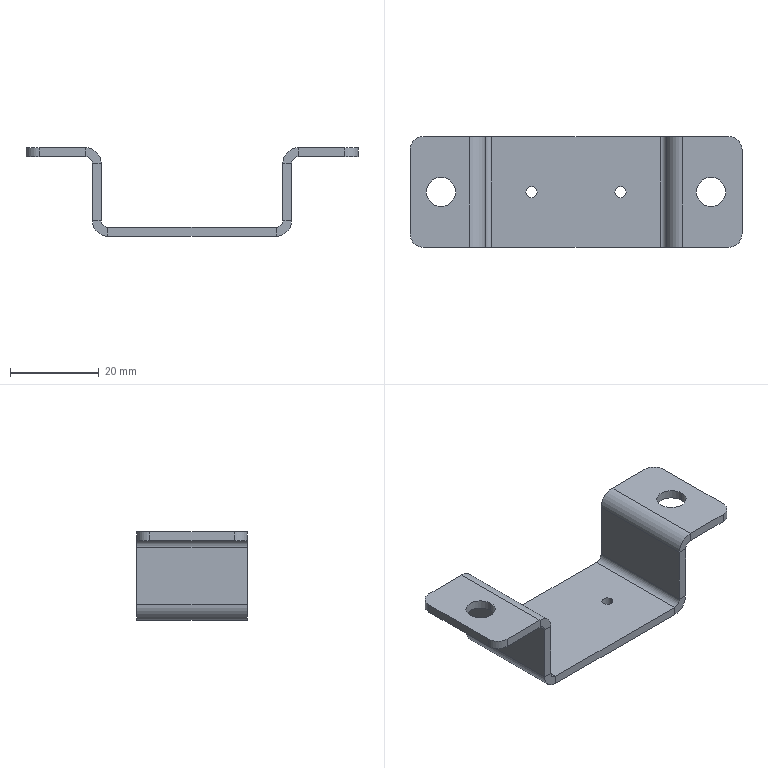Part | STEP file | 16-Photoeye mounting plate | 1 solid | 50 faces | box 75 x 25 x 20 mm | volume 5163 mm3 | plane 30 | cylinder 20 | commonest cylinder face diameters 2.5 x4 3 x4 6 x4 6.6 x4 7 x4